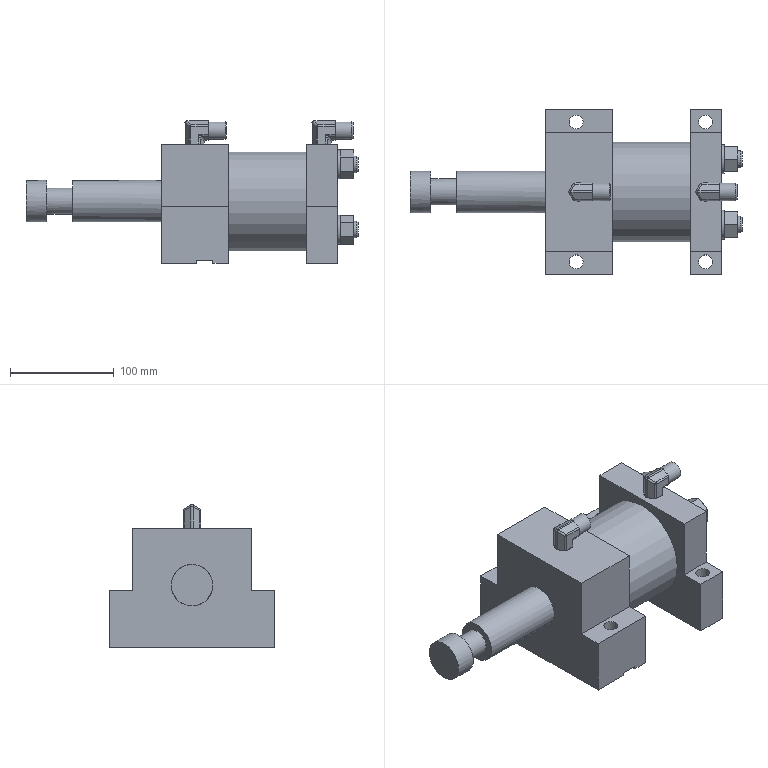Part | STEP file | solid 99 | 1 solid | 233 faces | box 320.319 x 160 x 137.691 mm | volume 2188173 mm3 | plane 138 | cylinder 64 | cone 20 | sphere 6 | spline 5 | commonest cylinder face diameters 4 x30 8 x12 13.5 x4 16 x4 17 x4 28 x4